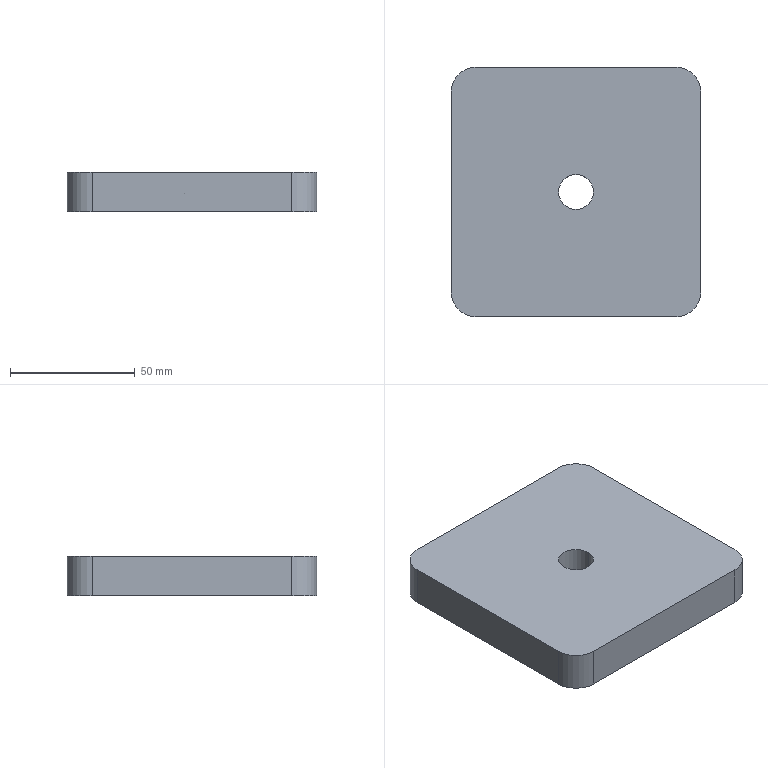Part | SolidWorks | features BaseBody 1 | 1 solid | 12 faces | box 100 x 100 x 16 mm | volume 156164 mm3 | cylinder 6 | plane 6 | commonest cylinder face diameters 20 x4 14 x2
STEP:
#1=CARTESIAN_POINT('',(7.,0.,16.));
#2=VERTEX_POINT('',#1);
#3=CARTESIAN_POINT('',(-7.,0.,16.));
#4=VERTEX_POINT('',#3);
#5=CARTESIAN_POINT('',(0.,0.,16.));
#6=DIRECTION('',(0.,0.,-1.));
#7=DIRECTION('',(-1.,0.,0.));
#8=AXIS2_PLACEMENT_3D('',#5,#6,#7);
#9=CIRCLE('',#8,7.);
#10=EDGE_CURVE('',#2,#4,#9,.T.);
#11=ORIENTED_EDGE('',*,*,#10,.F.);
#12=CARTESIAN_POINT('',(7.,0.,0.));
#13=VERTEX_POINT('',#12);
#14=CARTESIAN_POINT('',(7.,0.,16.));
#15=DIRECTION('',(0.,0.,-1.));
#16=VECTOR('',#15,1000.);
#17=LINE('',#14,#16);
#18=EDGE_CURVE('',#2,#13,#17,.T.);
#19=ORIENTED_EDGE('',*,*,#18,.T.);
#20=CARTESIAN_POINT('',(-7.,0.,0.));
#21=VERTEX_POINT('',#20);
#22=CARTESIAN_POINT('',(0.,0.,0.));
#23=DIRECTION('',(0.,0.,1.));
#24=DIRECTION('',(-1.,0.,0.));
#25=AXIS2_PLACEMENT_3D('',#22,#23,#24);
#26=CIRCLE('',#25,7.);
#27=EDGE_CURVE('',#21,#13,#26,.T.);
#28=ORIENTED_EDGE('',*,*,#27,.F.);
#29=CARTESIAN_POINT('',(-7.,0.,16.));
#30=DIRECTION('',(0.,0.,-1.));
#31=VECTOR('',#30,1000.);
#32=LINE('',#29,#31);
#33=EDGE_CURVE('',#4,#21,#32,.T.);
#34=ORIENTED_EDGE('',*,*,#33,.F.);
#35=EDGE_LOOP('',(#11,#19,#28,#34));
#36=FACE_OUTER_BOUND('',#35,.T.);
#37=CARTESIAN_POINT('',(0.,0.,16.));
#38=DIRECTION('',(0.,0.,-1.));
#39=DIRECTION('',(-1.,0.,0.));
#40=AXIS2_PLACEMENT_3D('',#37,#38,#39);
#41=CYLINDRICAL_SURFACE('',#40,7.);
#42=ADVANCED_FACE('',(#36),#41,.F.);
#43=ORIENTED_EDGE('',*,*,#27,.T.);
#44=CARTESIAN_POINT('',(0.,0.,0.));
#45=DIRECTION('',(0.,0.,1.));
#46=DIRECTION('',(-1.,0.,0.));
#47=AXIS2_PLACEMENT_3D('',#44,#45,#46);
#48=CIRCLE('',#47,7.);
#49=EDGE_CURVE('',#13,#21,#48,.T.);
#50=ORIENTED_EDGE('',*,*,#49,.T.);
#51=EDGE_LOOP('',(#43,#50));
#52=FACE_BOUND('',#51,.T.);
#53=CARTESIAN_POINT('',(-40.,50.,0.));
#54=VERTEX_POINT('',#53);
#55=CARTESIAN_POINT('',(40.,50.,0.));
#56=VERTEX_POINT('',#55);
#57=CARTESIAN_POINT('',(0.,50.,0.));
#58=DIRECTION('',(1.,0.,0.));
#59=VECTOR('',#58,1000.);
#60=LINE('',#57,#59);
#61=EDGE_CURVE('',#54,#56,#60,.T.);
#62=ORIENTED_EDGE('',*,*,#61,.T.);
#63=CARTESIAN_POINT('',(50.,40.,0.));
#64=VERTEX_POINT('',#63);
#65=CARTESIAN_POINT('',(40.,40.,0.));
#66=DIRECTION('',(0.,0.,-1.));
#67=DIRECTION('',(-1.,0.,0.));
#68=AXIS2_PLACEMENT_3D('',#65,#66,#67);
#69=CIRCLE('',#68,10.);
#70=EDGE_CURVE('',#56,#64,#69,.T.);
#71=ORIENTED_EDGE('',*,*,#70,.T.);
#72=CARTESIAN_POINT('',(50.,-40.,0.));
#73=VERTEX_POINT('',#72);
#74=CARTESIAN_POINT('',(50.,0.,0.));
#75=DIRECTION('',(0.,-1.,0.));
#76=VECTOR('',#75,1000.);
#77=LINE('',#74,#76);
#78=EDGE_CURVE('',#64,#73,#77,.T.);
#79=ORIENTED_EDGE('',*,*,#78,.T.);
#80=CARTESIAN_POINT('',(40.,-50.,0.));
#81=VERTEX_POINT('',#80);
#82=CARTESIAN_POINT('',(40.,-40.,0.));
#83=DIRECTION('',(0.,0.,-1.));
#84=DIRECTION('',(-1.,0.,0.));
#85=AXIS2_PLACEMENT_3D('',#82,#83,#84);
#86=CIRCLE('',#85,10.);
#87=EDGE_CURVE('',#73,#81,#86,.T.);
#88=ORIENTED_EDGE('',*,*,#87,.T.);
#89=CARTESIAN_POINT('',(-40.,-50.,0.));
#90=VERTEX_POINT('',#89);
#91=CARTESIAN_POINT('',(0.,-50.,0.));
#92=DIRECTION('',(-1.,0.,0.));
#93=VECTOR('',#92,1000.);
#94=LINE('',#91,#93);
#95=EDGE_CURVE('',#81,#90,#94,.T.);
#96=ORIENTED_EDGE('',*,*,#95,.T.);
#97=CARTESIAN_POINT('',(-50.,-40.,0.));
#98=VERTEX_POINT('',#97);
#99=CARTESIAN_POINT('',(-40.,-40.,0.));
#100=DIRECTION('',(0.,0.,-1.));
#101=DIRECTION('',(-1.,0.,0.));
#102=AXIS2_PLACEMENT_3D('',#99,#100,#101);
#103=CIRCLE('',#102,10.);
#104=EDGE_CURVE('',#90,#98,#103,.T.);
#105=ORIENTED_EDGE('',*,*,#104,.T.);
#106=CARTESIAN_POINT('',(-50.,40.,0.));
#107=VERTEX_POINT('',#106);
#108=CARTESIAN_POINT('',(-50.,0.,0.));
#109=DIRECTION('',(0.,1.,0.));
#110=VECTOR('',#109,1000.);
#111=LINE('',#108,#110);
#112=EDGE_CURVE('',#98,#107,#111,.T.);
#113=ORIENTED_EDGE('',*,*,#112,.T.);
#114=CARTESIAN_POINT('',(-40.,40.,0.));
#115=DIRECTION('',(0.,0.,-1.));
#116=DIRECTION('',(-1.,0.,0.));
#117=AXIS2_PLACEMENT_3D('',#114,#115,#116);
#118=CIRCLE('',#117,10.);
#119=EDGE_CURVE('',#107,#54,#118,.T.);
#120=ORIENTED_EDGE('',*,*,#119,.T.);
#121=EDGE_LOOP('',(#62,#71,#79,#88,#96,#105,#113,#120));
#122=FACE_OUTER_BOUND('',#121,.T.);
#123=CARTESIAN_POINT('',(0.,0.,0.));
#124=DIRECTION('',(0.,0.,-1.));
#125=DIRECTION('',(-1.,0.,0.));
#126=AXIS2_PLACEMENT_3D('',#123,#124,#125);
#127=PLANE('',#126);
#128=ADVANCED_FACE('',(#52,#122),#127,.T.);
#129=ORIENTED_EDGE('',*,*,#18,.F.);
#130=CARTESIAN_POINT('',(0.,0.,16.));
#131=DIRECTION('',(0.,0.,-1.));
#132=DIRECTION('',(-1.,0.,0.));
#133=AXIS2_PLACEMENT_3D('',#130,#131,#132);
#134=CIRCLE('',#133,7.);
#135=EDGE_CURVE('',#4,#2,#134,.T.);
#136=ORIENTED_EDGE('',*,*,#135,.F.);
#137=ORIENTED_EDGE('',*,*,#33,.T.);
#138=ORIENTED_EDGE('',*,*,#49,.F.);
#139=EDGE_LOOP('',(#129,#136,#137,#138));
#140=FACE_OUTER_BOUND('',#139,.T.);
#141=CARTESIAN_POINT('',(0.,0.,16.));
#142=DIRECTION('',(0.,0.,-1.));
#143=DIRECTION('',(-1.,0.,0.));
#144=AXIS2_PLACEMENT_3D('',#141,#142,#143);
#145=CYLINDRICAL_SURFACE('',#144,7.);
#146=ADVANCED_FACE('',(#140),#145,.F.);
#147=ORIENTED_EDGE('',*,*,#70,.F.);
#148=CARTESIAN_POINT('',(40.,50.,16.));
#149=VERTEX_POINT('',#148);
#150=CARTESIAN_POINT('',(40.,50.,16.));
#151=DIRECTION('',(0.,0.,1.));
#152=VECTOR('',#151,1000.);
#153=LINE('',#150,#152);
#154=EDGE_CURVE('',#56,#149,#153,.T.);
#155=ORIENTED_EDGE('',*,*,#154,.T.);
#156=CARTESIAN_POINT('',(50.,40.,16.));
#157=VERTEX_POINT('',#156);
#158=CARTESIAN_POINT('',(40.,40.,16.));
#159=DIRECTION('',(0.,0.,-1.));
#160=DIRECTION('',(-1.,0.,0.));
#161=AXIS2_PLACEMENT_3D('',#158,#159,#160);
#162=CIRCLE('',#161,10.);
#163=EDGE_CURVE('',#149,#157,#162,.T.);
#164=ORIENTED_EDGE('',*,*,#163,.T.);
#165=CARTESIAN_POINT('',(50.,40.,16.));
#166=DIRECTION('',(0.,0.,-1.));
#167=VECTOR('',#166,1000.);
#168=LINE('',#165,#167);
#169=EDGE_CURVE('',#157,#64,#168,.T.);
#170=ORIENTED_EDGE('',*,*,#169,.T.);
#171=EDGE_LOOP('',(#147,#155,#164,#170));
#172=FACE_OUTER_BOUND('',#171,.T.);
#173=CARTESIAN_POINT('',(40.,40.,16.));
#174=DIRECTION('',(0.,0.,-1.));
#175=DIRECTION('',(-1.,0.,0.));
#176=AXIS2_PLACEMENT_3D('',#173,#174,#175);
#177=CYLINDRICAL_SURFACE('',#176,10.);
#178=ADVANCED_FACE('',(#172),#177,.T.);
#179=CARTESIAN_POINT('',(-40.,50.,16.));
#180=VERTEX_POINT('',#179);
#181=CARTESIAN_POINT('',(-40.,50.,16.));
#182=DIRECTION('',(0.,0.,-1.));
#183=VECTOR('',#182,1000.);
#184=LINE('',#181,#183);
#185=EDGE_CURVE('',#180,#54,#184,.T.);
#186=ORIENTED_EDGE('',*,*,#185,.F.);
#187=CARTESIAN_POINT('',(50.,50.,16.));
#188=DIRECTION('',(-1.,0.,0.));
#189=VECTOR('',#188,1000.);
#190=LINE('',#187,#189);
#191=EDGE_CURVE('',#149,#180,#190,.T.);
#192=ORIENTED_EDGE('',*,*,#191,.F.);
#193=ORIENTED_EDGE('',*,*,#154,.F.);
#194=ORIENTED_EDGE('',*,*,#61,.F.);
#195=EDGE_LOOP('',(#186,#192,#193,#194));
#196=FACE_OUTER_BOUND('',#195,.T.);
#197=CARTESIAN_POINT('',(50.,50.,16.));
#198=DIRECTION('',(0.,-1.,0.));
#199=DIRECTION('',(1.,0.,0.));
#200=AXIS2_PLACEMENT_3D('',#197,#198,#199);
#201=PLANE('',#200);
#202=ADVANCED_FACE('',(#196),#201,.F.);
#203=ORIENTED_EDGE('',*,*,#119,.F.);
#204=CARTESIAN_POINT('',(-50.,40.,16.));
#205=VERTEX_POINT('',#204);
#206=CARTESIAN_POINT('',(-50.,40.,16.));
#207=DIRECTION('',(0.,0.,1.));
#208=VECTOR('',#207,1000.);
#209=LINE('',#206,#208);
#210=EDGE_CURVE('',#107,#205,#209,.T.);
#211=ORIENTED_EDGE('',*,*,#210,.T.);
#212=CARTESIAN_POINT('',(-40.,40.,16.));
#213=DIRECTION('',(0.,0.,-1.));
#214=DIRECTION('',(-1.,0.,0.));
#215=AXIS2_PLACEMENT_3D('',#212,#213,#214);
#216=CIRCLE('',#215,10.);
#217=EDGE_CURVE('',#205,#180,#216,.T.);
#218=ORIENTED_EDGE('',*,*,#217,.T.);
#219=ORIENTED_EDGE('',*,*,#185,.T.);
#220=EDGE_LOOP('',(#203,#211,#218,#219));
#221=FACE_OUTER_BOUND('',#220,.T.);
#222=CARTESIAN_POINT('',(-40.,40.,16.));
#223=DIRECTION('',(0.,0.,-1.));
#224=DIRECTION('',(-1.,0.,0.));
#225=AXIS2_PLACEMENT_3D('',#222,#223,#224);
#226=CYLINDRICAL_SURFACE('',#225,10.);
#227=ADVANCED_FACE('',(#221),#226,.T.);
#228=CARTESIAN_POINT('',(-50.,-40.,16.));
#229=VERTEX_POINT('',#228);
#230=CARTESIAN_POINT('',(-50.,-40.,16.));
#231=DIRECTION('',(0.,0.,-1.));
#232=VECTOR('',#231,1000.);
#233=LINE('',#230,#232);
#234=EDGE_CURVE('',#229,#98,#233,.T.);
#235=ORIENTED_EDGE('',*,*,#234,.F.);
#236=CARTESIAN_POINT('',(-50.,50.,16.));
#237=DIRECTION('',(0.,-1.,0.));
#238=VECTOR('',#237,1000.);
#239=LINE('',#236,#238);
#240=EDGE_CURVE('',#205,#229,#239,.T.);
#241=ORIENTED_EDGE('',*,*,#240,.F.);
#242=ORIENTED_EDGE('',*,*,#210,.F.);
#243=ORIENTED_EDGE('',*,*,#112,.F.);
#244=EDGE_LOOP('',(#235,#241,#242,#243));
#245=FACE_OUTER_BOUND('',#244,.T.);
#246=CARTESIAN_POINT('',(-50.,50.,16.));
#247=DIRECTION('',(1.,0.,0.));
#248=DIRECTION('',(0.,1.,0.));
#249=AXIS2_PLACEMENT_3D('',#246,#247,#248);
#250=PLANE('',#249);
#251=ADVANCED_FACE('',(#245),#250,.F.);
#252=ORIENTED_EDGE('',*,*,#104,.F.);
#253=CARTESIAN_POINT('',(-40.,-50.,16.));
#254=VERTEX_POINT('',#253);
#255=CARTESIAN_POINT('',(-40.,-50.,16.));
#256=DIRECTION('',(0.,0.,1.));
#257=VECTOR('',#256,1000.);
#258=LINE('',#255,#257);
#259=EDGE_CURVE('',#90,#254,#258,.T.);
#260=ORIENTED_EDGE('',*,*,#259,.T.);
#261=CARTESIAN_POINT('',(-40.,-40.,16.));
#262=DIRECTION('',(0.,0.,-1.));
#263=DIRECTION('',(-1.,0.,0.));
#264=AXIS2_PLACEMENT_3D('',#261,#262,#263);
#265=CIRCLE('',#264,10.);
#266=EDGE_CURVE('',#254,#229,#265,.T.);
#267=ORIENTED_EDGE('',*,*,#266,.T.);
#268=ORIENTED_EDGE('',*,*,#234,.T.);
#269=EDGE_LOOP('',(#252,#260,#267,#268));
#270=FACE_OUTER_BOUND('',#269,.T.);
#271=CARTESIAN_POINT('',(-40.,-40.,16.));
#272=DIRECTION('',(0.,0.,-1.));
#273=DIRECTION('',(-1.,0.,0.));
#274=AXIS2_PLACEMENT_3D('',#271,#272,#273);
#275=CYLINDRICAL_SURFACE('',#274,10.);
#276=ADVANCED_FACE('',(#270),#275,.T.);
#277=CARTESIAN_POINT('',(40.,-50.,16.));
#278=VERTEX_POINT('',#277);
#279=CARTESIAN_POINT('',(40.,-50.,16.));
#280=DIRECTION('',(0.,0.,-1.));
#281=VECTOR('',#280,1000.);
#282=LINE('',#279,#281);
#283=EDGE_CURVE('',#278,#81,#282,.T.);
#284=ORIENTED_EDGE('',*,*,#283,.F.);
#285=CARTESIAN_POINT('',(50.,-50.,16.));
#286=DIRECTION('',(1.,0.,0.));
#287=VECTOR('',#286,1000.);
#288=LINE('',#285,#287);
#289=EDGE_CURVE('',#254,#278,#288,.T.);
#290=ORIENTED_EDGE('',*,*,#289,.F.);
#291=ORIENTED_EDGE('',*,*,#259,.F.);
#292=ORIENTED_EDGE('',*,*,#95,.F.);
#293=EDGE_LOOP('',(#284,#290,#291,#292));
#294=FACE_OUTER_BOUND('',#293,.T.);
#295=CARTESIAN_POINT('',(50.,-50.,16.));
#296=DIRECTION('',(0.,1.,0.));
#297=DIRECTION('',(-1.,0.,0.));
#298=AXIS2_PLACEMENT_3D('',#295,#296,#297);
#299=PLANE('',#298);
#300=ADVANCED_FACE('',(#294),#299,.F.);
#301=ORIENTED_EDGE('',*,*,#87,.F.);
#302=CARTESIAN_POINT('',(50.,-40.,16.));
#303=VERTEX_POINT('',#302);
#304=CARTESIAN_POINT('',(50.,-40.,16.));
#305=DIRECTION('',(0.,0.,1.));
#306=VECTOR('',#305,1000.);
#307=LINE('',#304,#306);
#308=EDGE_CURVE('',#73,#303,#307,.T.);
#309=ORIENTED_EDGE('',*,*,#308,.T.);
#310=CARTESIAN_POINT('',(40.,-40.,16.));
#311=DIRECTION('',(0.,0.,-1.));
#312=DIRECTION('',(-1.,0.,0.));
#313=AXIS2_PLACEMENT_3D('',#310,#311,#312);
#314=CIRCLE('',#313,10.);
#315=EDGE_CURVE('',#303,#278,#314,.T.);
#316=ORIENTED_EDGE('',*,*,#315,.T.);
#317=ORIENTED_EDGE('',*,*,#283,.T.);
#318=EDGE_LOOP('',(#301,#309,#316,#317));
#319=FACE_OUTER_BOUND('',#318,.T.);
#320=CARTESIAN_POINT('',(40.,-40.,16.));
#321=DIRECTION('',(0.,0.,-1.));
#322=DIRECTION('',(-1.,0.,0.));
#323=AXIS2_PLACEMENT_3D('',#320,#321,#322);
#324=CYLINDRICAL_SURFACE('',#323,10.);
#325=ADVANCED_FACE('',(#319),#324,.T.);
#326=ORIENTED_EDGE('',*,*,#308,.F.);
#327=ORIENTED_EDGE('',*,*,#78,.F.);
#328=ORIENTED_EDGE('',*,*,#169,.F.);
#329=CARTESIAN_POINT('',(50.,50.,16.));
#330=DIRECTION('',(0.,1.,0.));
#331=VECTOR('',#330,1000.);
#332=LINE('',#329,#331);
#333=EDGE_CURVE('',#303,#157,#332,.T.);
#334=ORIENTED_EDGE('',*,*,#333,.F.);
#335=EDGE_LOOP('',(#326,#327,#328,#334));
#336=FACE_OUTER_BOUND('',#335,.T.);
#337=CARTESIAN_POINT('',(50.,50.,16.));
#338=DIRECTION('',(-1.,0.,0.));
#339=DIRECTION('',(0.,-1.,0.));
#340=AXIS2_PLACEMENT_3D('',#337,#338,#339);
#341=PLANE('',#340);
#342=ADVANCED_FACE('',(#336),#341,.F.);
#343=ORIENTED_EDGE('',*,*,#135,.T.);
#344=ORIENTED_EDGE('',*,*,#10,.T.);
#345=EDGE_LOOP('',(#343,#344));
#346=FACE_BOUND('',#345,.T.);
#347=ORIENTED_EDGE('',*,*,#315,.F.);
#348=ORIENTED_EDGE('',*,*,#333,.T.);
#349=ORIENTED_EDGE('',*,*,#163,.F.);
#350=ORIENTED_EDGE('',*,*,#191,.T.);
#351=ORIENTED_EDGE('',*,*,#217,.F.);
#352=ORIENTED_EDGE('',*,*,#240,.T.);
#353=ORIENTED_EDGE('',*,*,#266,.F.);
#354=ORIENTED_EDGE('',*,*,#289,.T.);
#355=EDGE_LOOP('',(#347,#348,#349,#350,#351,#352,#353,#354));
#356=FACE_OUTER_BOUND('',#355,.T.);
#357=CARTESIAN_POINT('',(0.,0.,16.));
#358=DIRECTION('',(0.,0.,-1.));
#359=DIRECTION('',(-1.,0.,0.));
#360=AXIS2_PLACEMENT_3D('',#357,#358,#359);
#361=PLANE('',#360);
#362=ADVANCED_FACE('',(#346,#356),#361,.F.);
#363=CLOSED_SHELL('',(#42,#128,#146,#178,#202,#227,#251,#276,#300,#325,#342,#362));
#364=MANIFOLD_SOLID_BREP('',#363);
#365=CARTESIAN_POINT('',(0.,0.,0.));
#366=DIRECTION('',(0.,0.,1.));
#367=DIRECTION('',(1.,0.,0.));
#368=AXIS2_PLACEMENT_3D('',#365,#366,#367);
#369=(LENGTH_UNIT()NAMED_UNIT(*)SI_UNIT(.MILLI.,.METRE.));
#370=UNCERTAINTY_MEASURE_WITH_UNIT(LENGTH_MEASURE(0.00001),#369,'','');
#371=(NAMED_UNIT(*)PLANE_ANGLE_UNIT()SI_UNIT($,.RADIAN.));
#372=(NAMED_UNIT(*)SI_UNIT($,.STERADIAN.)SOLID_ANGLE_UNIT());
#373=(GEOMETRIC_REPRESENTATION_CONTEXT(3)GLOBAL_UNCERTAINTY_ASSIGNED_CONTEXT((#370))GLOBAL_UNIT_ASSIGNED_CONTEXT((#369,#371,#372))REPRESENTATION_CONTEXT('',''));
#374=ADVANCED_BREP_SHAPE_REPRESENTATION('',(#364,#368),#373);